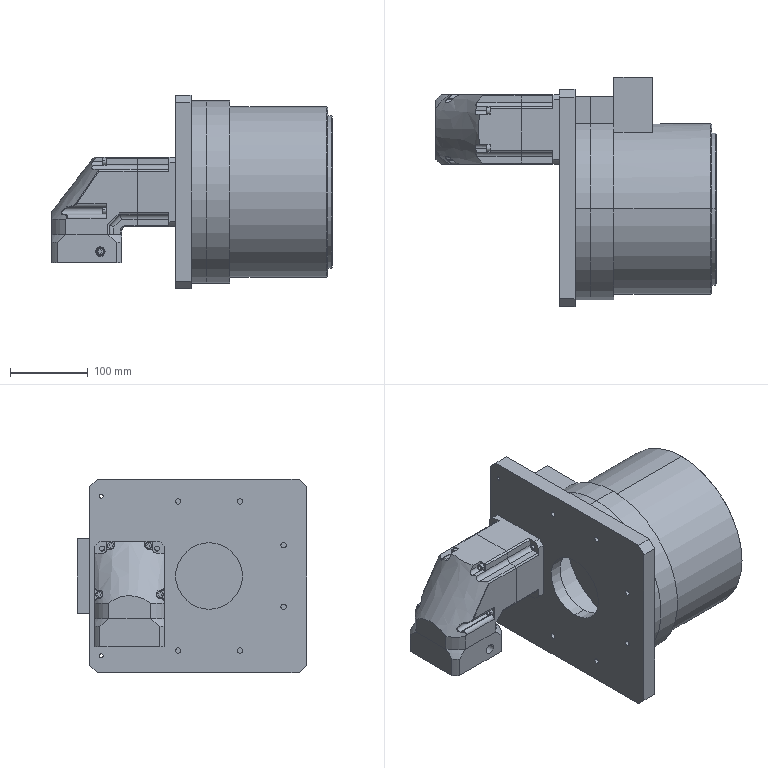Part | 17 solids | 712 faces | box 361.5 x 296 x 250 mm | volume 9686499 mm3 | cylinder 351 | plane 208 | cone 78 | spline 75 | commonest cylinder face diameters 6.8 x50 5 x44 10 x37 105 x24 4.2 x16 11 x15